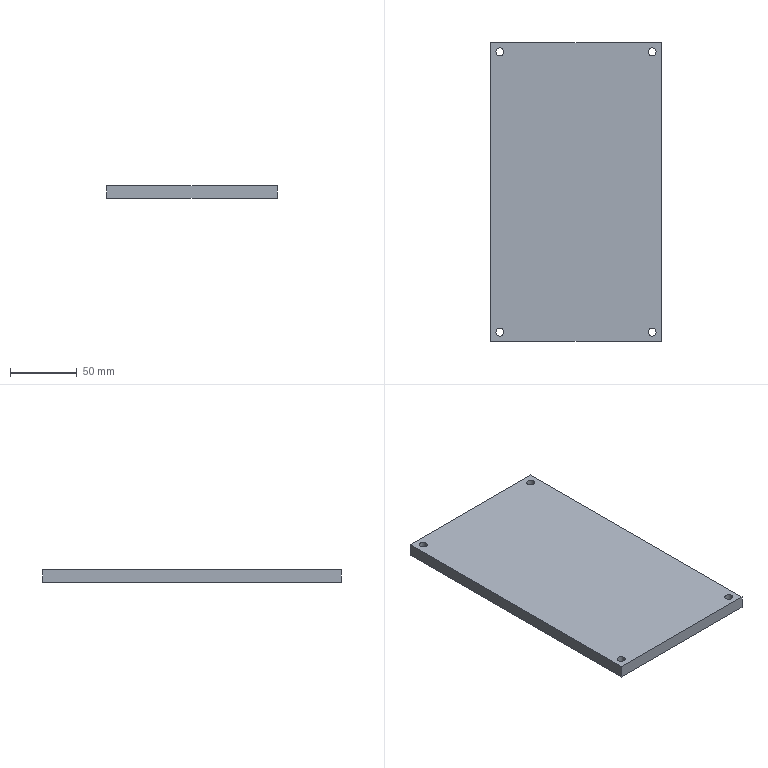Part | NX | features DATUM_CSYS 1, EXTRACT_DATUM_PLANE 1, EXTRUDE 1, SKETCH 1 | 1 solid | 10 faces | box 128 x 224 x 9.5 mm | volume 271310 mm3 | plane 6 | cylinder 4 | commonest cylinder face diameters 6 x4
STEP:
#1=CARTESIAN_POINT('',(-64.,112.,9.5));
#2=VERTEX_POINT('',#1);
#3=CARTESIAN_POINT('',(-64.,-112.,9.5));
#4=VERTEX_POINT('',#3);
#5=CARTESIAN_POINT('',(-64.,112.,9.5));
#6=DIRECTION('',(0.,-1.,0.));
#7=VECTOR('',#6,1000.);
#8=LINE('',#5,#7);
#9=EDGE_CURVE('',#2,#4,#8,.T.);
#10=ORIENTED_EDGE('',*,*,#9,.F.);
#11=CARTESIAN_POINT('',(-64.,112.,0.));
#12=VERTEX_POINT('',#11);
#13=CARTESIAN_POINT('',(-64.,112.,0.));
#14=DIRECTION('',(0.,0.,1.));
#15=VECTOR('',#14,1000.);
#16=LINE('',#13,#15);
#17=EDGE_CURVE('',#12,#2,#16,.T.);
#18=ORIENTED_EDGE('',*,*,#17,.F.);
#19=CARTESIAN_POINT('',(-64.,-112.,0.));
#20=VERTEX_POINT('',#19);
#21=CARTESIAN_POINT('',(-64.,112.,0.));
#22=DIRECTION('',(0.,-1.,0.));
#23=VECTOR('',#22,1000.);
#24=LINE('',#21,#23);
#25=EDGE_CURVE('',#12,#20,#24,.T.);
#26=ORIENTED_EDGE('',*,*,#25,.T.);
#27=CARTESIAN_POINT('',(-64.,-112.,0.));
#28=DIRECTION('',(0.,0.,1.));
#29=VECTOR('',#28,1000.);
#30=LINE('',#27,#29);
#31=EDGE_CURVE('',#20,#4,#30,.T.);
#32=ORIENTED_EDGE('',*,*,#31,.T.);
#33=EDGE_LOOP('',(#10,#18,#26,#32));
#34=FACE_BOUND('',#33,.T.);
#35=CARTESIAN_POINT('',(-64.,112.,0.));
#36=DIRECTION('',(-1.,0.,0.));
#37=DIRECTION('',(0.,0.,1.));
#38=AXIS2_PLACEMENT_3D('',#35,#36,#37);
#39=PLANE('',#38);
#40=ADVANCED_FACE('',(#34),#39,.T.);
#41=CARTESIAN_POINT('',(64.,-112.,9.5));
#42=VERTEX_POINT('',#41);
#43=CARTESIAN_POINT('',(-64.,-112.,9.5));
#44=DIRECTION('',(1.,0.,0.));
#45=VECTOR('',#44,1000.);
#46=LINE('',#43,#45);
#47=EDGE_CURVE('',#4,#42,#46,.T.);
#48=ORIENTED_EDGE('',*,*,#47,.F.);
#49=ORIENTED_EDGE('',*,*,#31,.F.);
#50=CARTESIAN_POINT('',(64.,-112.,0.));
#51=VERTEX_POINT('',#50);
#52=CARTESIAN_POINT('',(-64.,-112.,0.));
#53=DIRECTION('',(1.,0.,0.));
#54=VECTOR('',#53,1000.);
#55=LINE('',#52,#54);
#56=EDGE_CURVE('',#20,#51,#55,.T.);
#57=ORIENTED_EDGE('',*,*,#56,.T.);
#58=CARTESIAN_POINT('',(64.,-112.,0.));
#59=DIRECTION('',(0.,0.,1.));
#60=VECTOR('',#59,1000.);
#61=LINE('',#58,#60);
#62=EDGE_CURVE('',#51,#42,#61,.T.);
#63=ORIENTED_EDGE('',*,*,#62,.T.);
#64=EDGE_LOOP('',(#48,#49,#57,#63));
#65=FACE_BOUND('',#64,.T.);
#66=CARTESIAN_POINT('',(-64.,-112.,0.));
#67=DIRECTION('',(0.,-1.,0.));
#68=DIRECTION('',(0.,0.,-1.));
#69=AXIS2_PLACEMENT_3D('',#66,#67,#68);
#70=PLANE('',#69);
#71=ADVANCED_FACE('',(#65),#70,.T.);
#72=CARTESIAN_POINT('',(64.,112.,9.5));
#73=VERTEX_POINT('',#72);
#74=CARTESIAN_POINT('',(64.,-112.,9.5));
#75=DIRECTION('',(0.,1.,0.));
#76=VECTOR('',#75,1000.);
#77=LINE('',#74,#76);
#78=EDGE_CURVE('',#42,#73,#77,.T.);
#79=ORIENTED_EDGE('',*,*,#78,.F.);
#80=ORIENTED_EDGE('',*,*,#62,.F.);
#81=CARTESIAN_POINT('',(64.,112.,0.));
#82=VERTEX_POINT('',#81);
#83=CARTESIAN_POINT('',(64.,-112.,0.));
#84=DIRECTION('',(0.,1.,0.));
#85=VECTOR('',#84,1000.);
#86=LINE('',#83,#85);
#87=EDGE_CURVE('',#51,#82,#86,.T.);
#88=ORIENTED_EDGE('',*,*,#87,.T.);
#89=CARTESIAN_POINT('',(64.,112.,0.));
#90=DIRECTION('',(0.,0.,1.));
#91=VECTOR('',#90,1000.);
#92=LINE('',#89,#91);
#93=EDGE_CURVE('',#82,#73,#92,.T.);
#94=ORIENTED_EDGE('',*,*,#93,.T.);
#95=EDGE_LOOP('',(#79,#80,#88,#94));
#96=FACE_BOUND('',#95,.T.);
#97=CARTESIAN_POINT('',(64.,-112.,0.));
#98=DIRECTION('',(1.,0.,0.));
#99=DIRECTION('',(0.,0.,-1.));
#100=AXIS2_PLACEMENT_3D('',#97,#98,#99);
#101=PLANE('',#100);
#102=ADVANCED_FACE('',(#96),#101,.T.);
#103=CARTESIAN_POINT('',(54.,-105.,9.5));
#104=VERTEX_POINT('',#103);
#105=CARTESIAN_POINT('',(57.,-105.,9.5));
#106=DIRECTION('',(0.,0.,-1.));
#107=DIRECTION('',(-1.,0.,0.));
#108=AXIS2_PLACEMENT_3D('',#105,#106,#107);
#109=CIRCLE('',#108,3.);
#110=EDGE_CURVE('',#104,#104,#109,.T.);
#111=ORIENTED_EDGE('',*,*,#110,.F.);
#112=EDGE_LOOP('',(#111));
#113=FACE_BOUND('',#112,.T.);
#114=CARTESIAN_POINT('',(60.,-105.,0.));
#115=VERTEX_POINT('',#114);
#116=CARTESIAN_POINT('',(57.,-105.,0.));
#117=DIRECTION('',(0.,0.,-1.));
#118=DIRECTION('',(1.,0.,0.));
#119=AXIS2_PLACEMENT_3D('',#116,#117,#118);
#120=CIRCLE('',#119,3.);
#121=EDGE_CURVE('',#115,#115,#120,.T.);
#122=ORIENTED_EDGE('',*,*,#121,.T.);
#123=EDGE_LOOP('',(#122));
#124=FACE_BOUND('',#123,.T.);
#125=CARTESIAN_POINT('',(57.,-105.,0.));
#126=DIRECTION('',(0.,0.,1.));
#127=DIRECTION('',(1.,0.,0.));
#128=AXIS2_PLACEMENT_3D('',#125,#126,#127);
#129=CYLINDRICAL_SURFACE('',#128,3.);
#130=ADVANCED_FACE('',(#113,#124),#129,.F.);
#131=CARTESIAN_POINT('',(-60.,105.,9.5));
#132=VERTEX_POINT('',#131);
#133=CARTESIAN_POINT('',(-57.,105.,9.5));
#134=DIRECTION('',(0.,0.,-1.));
#135=DIRECTION('',(-1.,0.,0.));
#136=AXIS2_PLACEMENT_3D('',#133,#134,#135);
#137=CIRCLE('',#136,3.);
#138=EDGE_CURVE('',#132,#132,#137,.T.);
#139=ORIENTED_EDGE('',*,*,#138,.F.);
#140=EDGE_LOOP('',(#139));
#141=FACE_BOUND('',#140,.T.);
#142=CARTESIAN_POINT('',(-54.,105.,0.));
#143=VERTEX_POINT('',#142);
#144=CARTESIAN_POINT('',(-57.,105.,0.));
#145=DIRECTION('',(0.,0.,-1.));
#146=DIRECTION('',(1.,0.,0.));
#147=AXIS2_PLACEMENT_3D('',#144,#145,#146);
#148=CIRCLE('',#147,3.);
#149=EDGE_CURVE('',#143,#143,#148,.T.);
#150=ORIENTED_EDGE('',*,*,#149,.T.);
#151=EDGE_LOOP('',(#150));
#152=FACE_BOUND('',#151,.T.);
#153=CARTESIAN_POINT('',(-57.,105.,0.));
#154=DIRECTION('',(0.,0.,1.));
#155=DIRECTION('',(1.,0.,0.));
#156=AXIS2_PLACEMENT_3D('',#153,#154,#155);
#157=CYLINDRICAL_SURFACE('',#156,3.);
#158=ADVANCED_FACE('',(#141,#152),#157,.F.);
#159=CARTESIAN_POINT('',(-60.,-105.,9.5));
#160=VERTEX_POINT('',#159);
#161=CARTESIAN_POINT('',(-57.,-105.,9.5));
#162=DIRECTION('',(0.,0.,-1.));
#163=DIRECTION('',(-1.,0.,0.));
#164=AXIS2_PLACEMENT_3D('',#161,#162,#163);
#165=CIRCLE('',#164,3.);
#166=EDGE_CURVE('',#160,#160,#165,.T.);
#167=ORIENTED_EDGE('',*,*,#166,.F.);
#168=EDGE_LOOP('',(#167));
#169=FACE_BOUND('',#168,.T.);
#170=CARTESIAN_POINT('',(-54.,-105.,0.));
#171=VERTEX_POINT('',#170);
#172=CARTESIAN_POINT('',(-57.,-105.,0.));
#173=DIRECTION('',(0.,0.,-1.));
#174=DIRECTION('',(1.,0.,0.));
#175=AXIS2_PLACEMENT_3D('',#172,#173,#174);
#176=CIRCLE('',#175,3.);
#177=EDGE_CURVE('',#171,#171,#176,.T.);
#178=ORIENTED_EDGE('',*,*,#177,.T.);
#179=EDGE_LOOP('',(#178));
#180=FACE_BOUND('',#179,.T.);
#181=CARTESIAN_POINT('',(-57.,-105.,0.));
#182=DIRECTION('',(0.,0.,1.));
#183=DIRECTION('',(1.,0.,0.));
#184=AXIS2_PLACEMENT_3D('',#181,#182,#183);
#185=CYLINDRICAL_SURFACE('',#184,3.);
#186=ADVANCED_FACE('',(#169,#180),#185,.F.);
#187=CARTESIAN_POINT('',(64.,112.,9.5));
#188=DIRECTION('',(-1.,0.,0.));
#189=VECTOR('',#188,1000.);
#190=LINE('',#187,#189);
#191=EDGE_CURVE('',#73,#2,#190,.T.);
#192=ORIENTED_EDGE('',*,*,#191,.F.);
#193=ORIENTED_EDGE('',*,*,#93,.F.);
#194=CARTESIAN_POINT('',(64.,112.,0.));
#195=DIRECTION('',(-1.,0.,0.));
#196=VECTOR('',#195,1000.);
#197=LINE('',#194,#196);
#198=EDGE_CURVE('',#82,#12,#197,.T.);
#199=ORIENTED_EDGE('',*,*,#198,.T.);
#200=ORIENTED_EDGE('',*,*,#17,.T.);
#201=EDGE_LOOP('',(#192,#193,#199,#200));
#202=FACE_BOUND('',#201,.T.);
#203=CARTESIAN_POINT('',(64.,112.,0.));
#204=DIRECTION('',(0.,1.,0.));
#205=DIRECTION('',(0.,0.,1.));
#206=AXIS2_PLACEMENT_3D('',#203,#204,#205);
#207=PLANE('',#206);
#208=ADVANCED_FACE('',(#202),#207,.T.);
#209=CARTESIAN_POINT('',(54.,105.,9.5));
#210=VERTEX_POINT('',#209);
#211=CARTESIAN_POINT('',(57.,105.,9.5));
#212=DIRECTION('',(0.,0.,-1.));
#213=DIRECTION('',(-1.,0.,0.));
#214=AXIS2_PLACEMENT_3D('',#211,#212,#213);
#215=CIRCLE('',#214,3.);
#216=EDGE_CURVE('',#210,#210,#215,.T.);
#217=ORIENTED_EDGE('',*,*,#216,.F.);
#218=EDGE_LOOP('',(#217));
#219=FACE_BOUND('',#218,.T.);
#220=CARTESIAN_POINT('',(60.,105.,0.));
#221=VERTEX_POINT('',#220);
#222=CARTESIAN_POINT('',(57.,105.,0.));
#223=DIRECTION('',(0.,0.,-1.));
#224=DIRECTION('',(1.,0.,0.));
#225=AXIS2_PLACEMENT_3D('',#222,#223,#224);
#226=CIRCLE('',#225,3.);
#227=EDGE_CURVE('',#221,#221,#226,.T.);
#228=ORIENTED_EDGE('',*,*,#227,.T.);
#229=EDGE_LOOP('',(#228));
#230=FACE_BOUND('',#229,.T.);
#231=CARTESIAN_POINT('',(57.,105.,0.));
#232=DIRECTION('',(0.,0.,1.));
#233=DIRECTION('',(1.,0.,0.));
#234=AXIS2_PLACEMENT_3D('',#231,#232,#233);
#235=CYLINDRICAL_SURFACE('',#234,3.);
#236=ADVANCED_FACE('',(#219,#230),#235,.F.);
#237=ORIENTED_EDGE('',*,*,#25,.F.);
#238=ORIENTED_EDGE('',*,*,#198,.F.);
#239=ORIENTED_EDGE('',*,*,#87,.F.);
#240=ORIENTED_EDGE('',*,*,#56,.F.);
#241=EDGE_LOOP('',(#237,#238,#239,#240));
#242=FACE_BOUND('',#241,.T.);
#243=ORIENTED_EDGE('',*,*,#177,.F.);
#244=EDGE_LOOP('',(#243));
#245=FACE_BOUND('',#244,.T.);
#246=ORIENTED_EDGE('',*,*,#149,.F.);
#247=EDGE_LOOP('',(#246));
#248=FACE_BOUND('',#247,.T.);
#249=ORIENTED_EDGE('',*,*,#121,.F.);
#250=EDGE_LOOP('',(#249));
#251=FACE_BOUND('',#250,.T.);
#252=ORIENTED_EDGE('',*,*,#227,.F.);
#253=EDGE_LOOP('',(#252));
#254=FACE_BOUND('',#253,.T.);
#255=CARTESIAN_POINT('',(-57.,-105.,0.));
#256=DIRECTION('',(0.,0.,-1.));
#257=DIRECTION('',(-1.,0.,0.));
#258=AXIS2_PLACEMENT_3D('',#255,#256,#257);
#259=PLANE('',#258);
#260=ADVANCED_FACE('',(#242,#245,#248,#251,#254),#259,.T.);
#261=ORIENTED_EDGE('',*,*,#9,.T.);
#262=ORIENTED_EDGE('',*,*,#47,.T.);
#263=ORIENTED_EDGE('',*,*,#78,.T.);
#264=ORIENTED_EDGE('',*,*,#191,.T.);
#265=EDGE_LOOP('',(#261,#262,#263,#264));
#266=FACE_BOUND('',#265,.T.);
#267=ORIENTED_EDGE('',*,*,#166,.T.);
#268=EDGE_LOOP('',(#267));
#269=FACE_BOUND('',#268,.T.);
#270=ORIENTED_EDGE('',*,*,#138,.T.);
#271=EDGE_LOOP('',(#270));
#272=FACE_BOUND('',#271,.T.);
#273=ORIENTED_EDGE('',*,*,#110,.T.);
#274=EDGE_LOOP('',(#273));
#275=FACE_BOUND('',#274,.T.);
#276=ORIENTED_EDGE('',*,*,#216,.T.);
#277=EDGE_LOOP('',(#276));
#278=FACE_BOUND('',#277,.T.);
#279=CARTESIAN_POINT('',(-57.,-105.,9.5));
#280=DIRECTION('',(0.,0.,-1.));
#281=DIRECTION('',(-1.,0.,0.));
#282=AXIS2_PLACEMENT_3D('',#279,#280,#281);
#283=PLANE('',#282);
#284=ADVANCED_FACE('',(#266,#269,#272,#275,#278),#283,.F.);
#285=CLOSED_SHELL('',(#40,#71,#102,#130,#158,#186,#208,#236,#260,#284));
#286=MANIFOLD_SOLID_BREP('',#285);
#287=(LENGTH_UNIT()NAMED_UNIT(*)SI_UNIT(.MILLI.,.METRE.));
#288=UNCERTAINTY_MEASURE_WITH_UNIT(LENGTH_MEASURE(0.00001),#287,'','');
#289=(NAMED_UNIT(*)PLANE_ANGLE_UNIT()SI_UNIT($,.RADIAN.));
#290=(NAMED_UNIT(*)SI_UNIT($,.STERADIAN.)SOLID_ANGLE_UNIT());
#291=(GEOMETRIC_REPRESENTATION_CONTEXT(3)GLOBAL_UNCERTAINTY_ASSIGNED_CONTEXT((#288))GLOBAL_UNIT_ASSIGNED_CONTEXT((#287,#289,#290))REPRESENTATION_CONTEXT('',''));
#292=ADVANCED_BREP_SHAPE_REPRESENTATION('',(#286),#291);